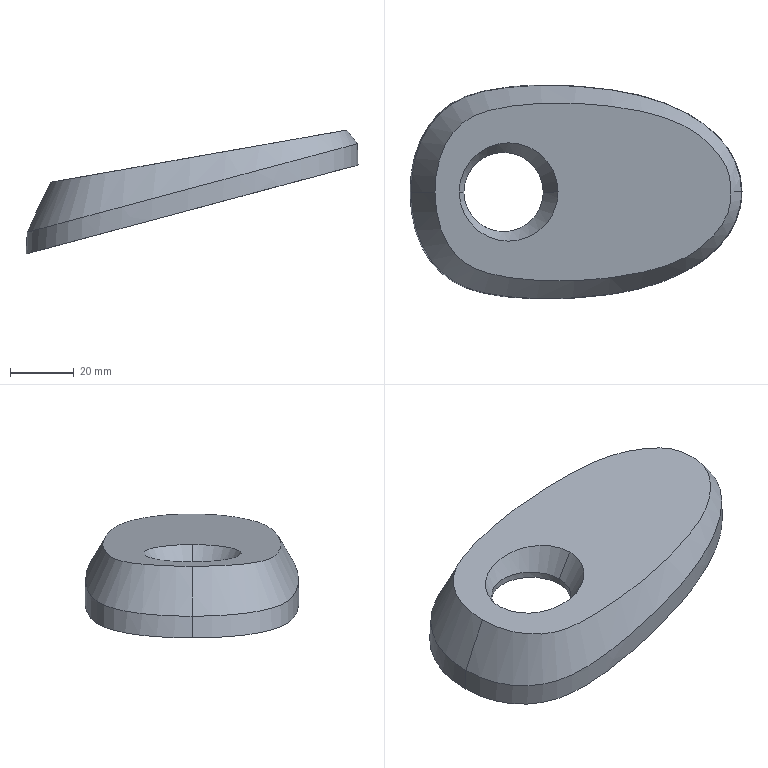Part | STEP file | 11-Cover31111 | 1 solid | 29 faces | box 105.323 x 67.359 x 38.98 mm | volume 17481 mm3 | spline 25 | plane 4